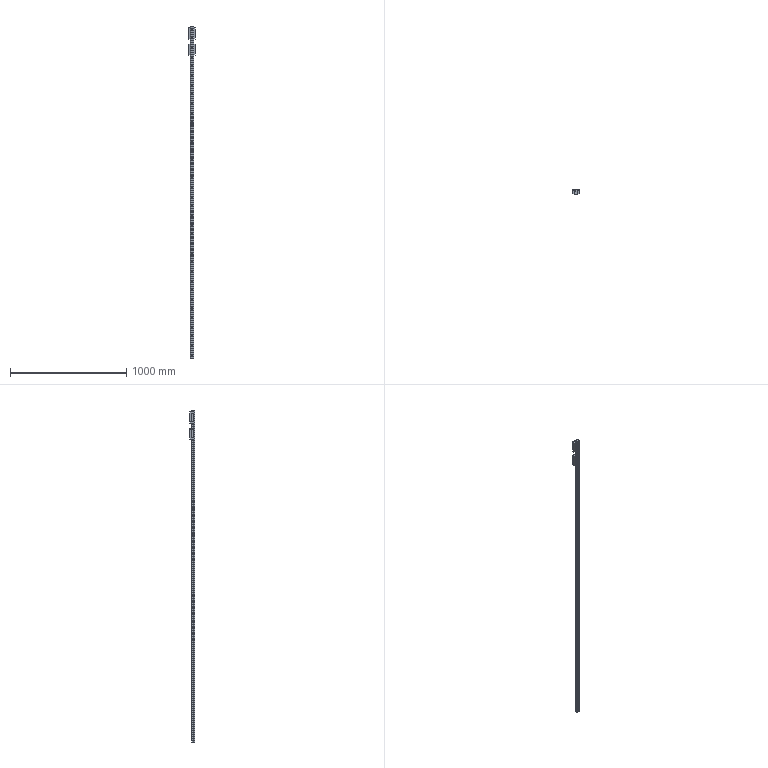Part | SolidWorks | 3 solids | 1012 faces | box 60 x 45 x 2850 mm | volume 1999576 mm3 | plane 670 | cylinder 222 | spline 120 | commonest cylinder face diameters 9 x72 14 x72 1.2 x36 8 x16 1.6 x14 5.66 x12